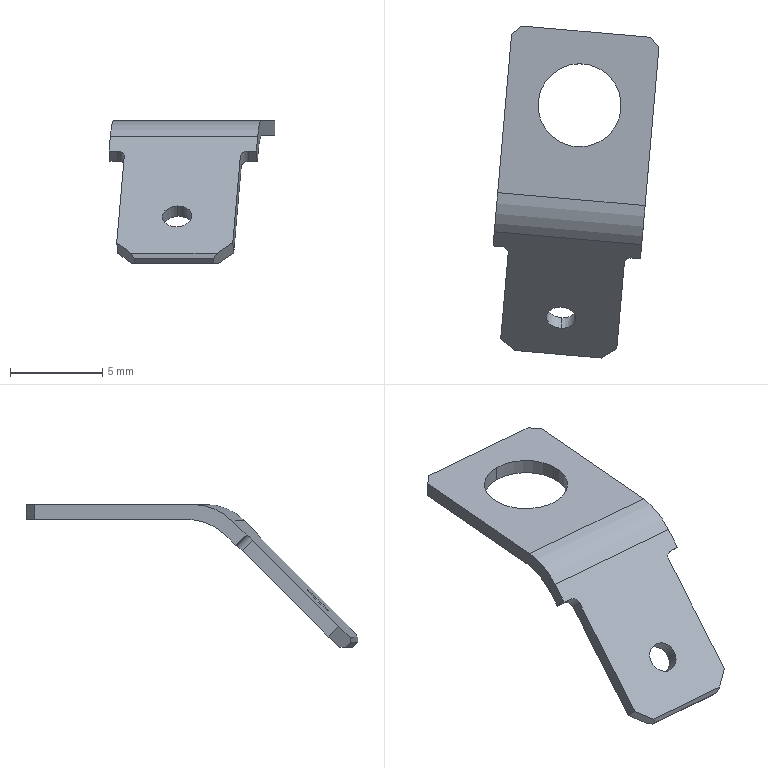Part | STEP file | MSBR-14_1_1_1_1 | 1 solid | 26 faces | box 8.97 x 17.939 x 7.73 mm | volume 103.786 mm3 | plane 18 | cylinder 8 | commonest cylinder face diameters 0.8 x2 1.6 x2 4.5 x2 6 x2
STEP:
#1=CARTESIAN_POINT('',(0.,0.,0.));
#2=DIRECTION('',(0.,0.,1.));
#3=DIRECTION('',(1.,0.,0.));
#4=AXIS2_PLACEMENT_3D('',#1,#2,#3);
#5=CARTESIAN_POINT('',(32.173,-29.923,38.));
#6=VERTEX_POINT('',#5);
#7=CARTESIAN_POINT('',(32.173,-29.923,38.8));
#8=VERTEX_POINT('',#7);
#9=CARTESIAN_POINT('',(32.173,-29.923,38.));
#10=DIRECTION('',(0.,0.,1.));
#11=VECTOR('',#10,0.8);
#12=LINE('',#9,#11);
#13=EDGE_CURVE('',#6,#8,#12,.T.);
#14=ORIENTED_EDGE('',*,*,#13,.F.);
#15=CARTESIAN_POINT('',(32.173,-34.423,38.));
#16=VERTEX_POINT('',#15);
#17=CARTESIAN_POINT('',(32.173,-32.173,38.));
#18=DIRECTION('',(0.,0.,-1.));
#19=DIRECTION('',(0.,-1.,0.));
#20=AXIS2_PLACEMENT_3D('',#17,#18,#19);
#21=CIRCLE('',#20,2.25);
#22=EDGE_CURVE('',#16,#6,#21,.T.);
#23=ORIENTED_EDGE('',*,*,#22,.F.);
#24=CARTESIAN_POINT('',(32.173,-34.423,38.8));
#25=VERTEX_POINT('',#24);
#26=CARTESIAN_POINT('',(32.173,-34.423,38.8));
#27=DIRECTION('',(0.,0.,-1.));
#28=VECTOR('',#27,0.8);
#29=LINE('',#26,#28);
#30=EDGE_CURVE('',#25,#16,#29,.T.);
#31=ORIENTED_EDGE('',*,*,#30,.F.);
#32=CARTESIAN_POINT('',(32.173,-32.173,38.8));
#33=DIRECTION('',(0.,0.,1.));
#34=DIRECTION('',(0.,1.,0.));
#35=AXIS2_PLACEMENT_3D('',#32,#33,#34);
#36=CIRCLE('',#35,2.25);
#37=EDGE_CURVE('',#8,#25,#36,.T.);
#38=ORIENTED_EDGE('',*,*,#37,.F.);
#39=EDGE_LOOP('',(#14,#23,#31,#38));
#40=FACE_OUTER_BOUND('',#39,.F.);
#41=CARTESIAN_POINT('',(32.173,-32.173,38.826));
#42=DIRECTION('',(0.,0.,-1.));
#43=DIRECTION('',(0.,-1.,0.));
#44=AXIS2_PLACEMENT_3D('',#41,#42,#43);
#45=CYLINDRICAL_SURFACE('',#44,2.25);
#46=ADVANCED_FACE('',(#40),#45,.F.);
#47=CARTESIAN_POINT('',(32.173,-32.173,38.));
#48=DIRECTION('',(0.,0.,-1.));
#49=DIRECTION('',(0.,1.,0.));
#50=AXIS2_PLACEMENT_3D('',#47,#48,#49);
#51=CIRCLE('',#50,2.25);
#52=EDGE_CURVE('',#6,#16,#51,.T.);
#53=ORIENTED_EDGE('',*,*,#52,.F.);
#54=ORIENTED_EDGE('',*,*,#13,.T.);
#55=CARTESIAN_POINT('',(32.173,-32.173,38.8));
#56=DIRECTION('',(0.,0.,1.));
#57=DIRECTION('',(0.,-1.,0.));
#58=AXIS2_PLACEMENT_3D('',#55,#56,#57);
#59=CIRCLE('',#58,2.25);
#60=EDGE_CURVE('',#25,#8,#59,.T.);
#61=ORIENTED_EDGE('',*,*,#60,.F.);
#62=ORIENTED_EDGE('',*,*,#30,.T.);
#63=EDGE_LOOP('',(#53,#54,#61,#62));
#64=FACE_OUTER_BOUND('',#63,.F.);
#65=CARTESIAN_POINT('',(32.173,-32.173,38.826));
#66=DIRECTION('',(0.,0.,-1.));
#67=DIRECTION('',(0.,1.,0.));
#68=AXIS2_PLACEMENT_3D('',#65,#66,#67);
#69=CYLINDRICAL_SURFACE('',#68,2.25);
#70=ADVANCED_FACE('',(#64),#69,.F.);
#71=CARTESIAN_POINT('',(35.744,-37.261,38.));
#72=VERTEX_POINT('',#71);
#73=CARTESIAN_POINT('',(27.774,-36.564,38.));
#74=VERTEX_POINT('',#73);
#75=CARTESIAN_POINT('',(35.744,-37.261,38.));
#76=DIRECTION('',(-0.9962,0.08716,0.));
#77=VECTOR('',#76,8.);
#78=LINE('',#75,#77);
#79=EDGE_CURVE('',#72,#74,#78,.T.);
#80=ORIENTED_EDGE('',*,*,#79,.F.);
#81=CARTESIAN_POINT('',(36.463,-29.035,38.));
#82=VERTEX_POINT('',#81);
#83=CARTESIAN_POINT('',(36.463,-29.035,38.));
#84=DIRECTION('',(-0.08716,-0.9962,0.));
#85=VECTOR('',#84,8.257);
#86=LINE('',#83,#85);
#87=EDGE_CURVE('',#82,#72,#86,.T.);
#88=ORIENTED_EDGE('',*,*,#87,.F.);
#89=CARTESIAN_POINT('',(36.009,-28.494,38.));
#90=VERTEX_POINT('',#89);
#91=CARTESIAN_POINT('',(36.463,-29.035,38.));
#92=DIRECTION('',(-0.6428,0.766,0.));
#93=VECTOR('',#92,0.7071);
#94=LINE('',#91,#93);
#95=EDGE_CURVE('',#82,#90,#94,.T.);
#96=ORIENTED_EDGE('',*,*,#95,.T.);
#97=CARTESIAN_POINT('',(29.035,-27.884,38.));
#98=VERTEX_POINT('',#97);
#99=CARTESIAN_POINT('',(29.035,-27.884,38.));
#100=DIRECTION('',(0.9962,-0.08716,0.));
#101=VECTOR('',#100,7.);
#102=LINE('',#99,#101);
#103=EDGE_CURVE('',#98,#90,#102,.T.);
#104=ORIENTED_EDGE('',*,*,#103,.F.);
#105=CARTESIAN_POINT('',(28.494,-28.338,38.));
#106=VERTEX_POINT('',#105);
#107=CARTESIAN_POINT('',(29.035,-27.884,38.));
#108=DIRECTION('',(-0.766,-0.6428,0.));
#109=VECTOR('',#108,0.7071);
#110=LINE('',#107,#109);
#111=EDGE_CURVE('',#98,#106,#110,.T.);
#112=ORIENTED_EDGE('',*,*,#111,.T.);
#113=CARTESIAN_POINT('',(27.774,-36.564,38.));
#114=DIRECTION('',(0.08716,0.9962,0.));
#115=VECTOR('',#114,8.257);
#116=LINE('',#113,#115);
#117=EDGE_CURVE('',#74,#106,#116,.T.);
#118=ORIENTED_EDGE('',*,*,#117,.F.);
#119=EDGE_LOOP('',(#80,#88,#96,#104,#112,#118));
#120=FACE_OUTER_BOUND('',#119,.F.);
#121=ORIENTED_EDGE('',*,*,#22,.T.);
#122=ORIENTED_EDGE('',*,*,#52,.T.);
#123=EDGE_LOOP('',(#121,#122));
#124=FACE_BOUND('',#123,.F.);
#125=CARTESIAN_POINT('',(32.14,-32.551,38.));
#126=DIRECTION('',(0.,0.,1.));
#127=DIRECTION('',(-0.08716,-0.9962,0.));
#128=AXIS2_PLACEMENT_3D('',#125,#126,#127);
#129=PLANE('',#128);
#130=ADVANCED_FACE('',(#120,#124),#129,.F.);
#131=ORIENTED_EDGE('',*,*,#79,.T.);
#132=CARTESIAN_POINT('',(27.589,-38.677,37.121));
#133=VERTEX_POINT('',#132);
#134=CARTESIAN_POINT('',(27.774,-36.564,35.));
#135=DIRECTION('',(-0.9962,0.08716,0.));
#136=DIRECTION('',(-0.06163,-0.7044,0.7071));
#137=AXIS2_PLACEMENT_3D('',#134,#135,#136);
#138=CIRCLE('',#137,3.);
#139=EDGE_CURVE('',#133,#74,#138,.T.);
#140=ORIENTED_EDGE('',*,*,#139,.F.);
#141=CARTESIAN_POINT('',(35.559,-39.374,37.121));
#142=VERTEX_POINT('',#141);
#143=CARTESIAN_POINT('',(27.589,-38.677,37.121));
#144=DIRECTION('',(0.9962,-0.08716,-0.000000002));
#145=VECTOR('',#144,8.);
#146=LINE('',#143,#145);
#147=EDGE_CURVE('',#133,#142,#146,.T.);
#148=ORIENTED_EDGE('',*,*,#147,.T.);
#149=CARTESIAN_POINT('',(35.744,-37.261,35.));
#150=DIRECTION('',(0.9962,-0.08716,0.));
#151=DIRECTION('',(0.000000003,0.000000023,1.));
#152=AXIS2_PLACEMENT_3D('',#149,#150,#151);
#153=CIRCLE('',#152,3.);
#154=EDGE_CURVE('',#72,#142,#153,.T.);
#155=ORIENTED_EDGE('',*,*,#154,.F.);
#156=EDGE_LOOP('',(#131,#140,#148,#155));
#157=FACE_OUTER_BOUND('',#156,.F.);
#158=CARTESIAN_POINT('',(35.903,-37.275,35.));
#159=DIRECTION('',(-0.9962,0.08716,0.));
#160=DIRECTION('',(-0.06163,-0.7044,0.7071));
#161=AXIS2_PLACEMENT_3D('',#158,#159,#160);
#162=CYLINDRICAL_SURFACE('',#161,3.);
#163=ADVANCED_FACE('',(#157),#162,.F.);
#164=CARTESIAN_POINT('',(27.745,-36.894,38.8));
#165=VERTEX_POINT('',#164);
#166=CARTESIAN_POINT('',(27.56,-39.007,37.921));
#167=VERTEX_POINT('',#166);
#168=CARTESIAN_POINT('',(27.745,-36.894,35.8));
#169=DIRECTION('',(0.9962,-0.08716,0.));
#170=DIRECTION('',(-0.000000002,-0.000000023,1.));
#171=AXIS2_PLACEMENT_3D('',#168,#169,#170);
#172=CIRCLE('',#171,3.);
#173=EDGE_CURVE('',#165,#167,#172,.T.);
#174=ORIENTED_EDGE('',*,*,#173,.T.);
#175=CARTESIAN_POINT('',(27.493,-39.774,37.151));
#176=VERTEX_POINT('',#175);
#177=CARTESIAN_POINT('',(27.56,-39.007,37.921));
#178=DIRECTION('',(-0.06163,-0.7044,-0.7071));
#179=VECTOR('',#178,1.089);
#180=LINE('',#177,#179);
#181=EDGE_CURVE('',#167,#176,#180,.T.);
#182=ORIENTED_EDGE('',*,*,#181,.T.);
#183=CARTESIAN_POINT('',(27.542,-39.211,36.586));
#184=VERTEX_POINT('',#183);
#185=CARTESIAN_POINT('',(27.493,-39.774,37.151));
#186=DIRECTION('',(0.06163,0.7044,-0.7071));
#187=VECTOR('',#186,0.8);
#188=LINE('',#185,#187);
#189=EDGE_CURVE('',#176,#184,#188,.T.);
#190=ORIENTED_EDGE('',*,*,#189,.T.);
#191=CARTESIAN_POINT('',(27.542,-39.211,36.586));
#192=DIRECTION('',(0.06163,0.7044,0.7071));
#193=VECTOR('',#192,0.7574);
#194=LINE('',#191,#193);
#195=EDGE_CURVE('',#184,#133,#194,.T.);
#196=ORIENTED_EDGE('',*,*,#195,.T.);
#197=ORIENTED_EDGE('',*,*,#139,.T.);
#198=ORIENTED_EDGE('',*,*,#117,.T.);
#199=CARTESIAN_POINT('',(28.494,-28.338,38.8));
#200=VERTEX_POINT('',#199);
#201=CARTESIAN_POINT('',(28.494,-28.338,38.8));
#202=DIRECTION('',(0.,0.,-1.));
#203=VECTOR('',#202,0.8);
#204=LINE('',#201,#203);
#205=EDGE_CURVE('',#200,#106,#204,.T.);
#206=ORIENTED_EDGE('',*,*,#205,.F.);
#207=CARTESIAN_POINT('',(27.745,-36.894,38.8));
#208=DIRECTION('',(0.08716,0.9962,0.));
#209=VECTOR('',#208,8.589);
#210=LINE('',#207,#209);
#211=EDGE_CURVE('',#165,#200,#210,.T.);
#212=ORIENTED_EDGE('',*,*,#211,.F.);
#213=EDGE_LOOP('',(#174,#182,#190,#196,#197,#198,#206,#212));
#214=FACE_OUTER_BOUND('',#213,.F.);
#215=CARTESIAN_POINT('',(27.993,-34.056,37.693));
#216=DIRECTION('',(0.9962,-0.08716,0.));
#217=DIRECTION('',(0.08716,0.9962,0.));
#218=AXIS2_PLACEMENT_3D('',#215,#216,#217);
#219=PLANE('',#218);
#220=ADVANCED_FACE('',(#214),#219,.F.);
#221=CARTESIAN_POINT('',(35.53,-39.705,37.921));
#222=VERTEX_POINT('',#221);
#223=CARTESIAN_POINT('',(35.715,-37.591,38.8));
#224=VERTEX_POINT('',#223);
#225=CARTESIAN_POINT('',(35.715,-37.591,35.8));
#226=DIRECTION('',(-0.9962,0.08716,0.));
#227=DIRECTION('',(-0.06163,-0.7044,0.7071));
#228=AXIS2_PLACEMENT_3D('',#225,#226,#227);
#229=CIRCLE('',#228,3.);
#230=EDGE_CURVE('',#222,#224,#229,.T.);
#231=ORIENTED_EDGE('',*,*,#230,.F.);
#232=CARTESIAN_POINT('',(35.53,-39.705,37.921));
#233=DIRECTION('',(-0.9962,0.08716,0.000000002));
#234=VECTOR('',#233,8.);
#235=LINE('',#232,#234);
#236=EDGE_CURVE('',#222,#167,#235,.T.);
#237=ORIENTED_EDGE('',*,*,#236,.T.);
#238=ORIENTED_EDGE('',*,*,#173,.F.);
#239=CARTESIAN_POINT('',(27.745,-36.894,38.8));
#240=DIRECTION('',(0.9962,-0.08716,0.));
#241=VECTOR('',#240,8.);
#242=LINE('',#239,#241);
#243=EDGE_CURVE('',#165,#224,#242,.T.);
#244=ORIENTED_EDGE('',*,*,#243,.T.);
#245=EDGE_LOOP('',(#231,#237,#238,#244));
#246=FACE_OUTER_BOUND('',#245,.F.);
#247=CARTESIAN_POINT('',(27.586,-36.88,35.8));
#248=DIRECTION('',(0.9962,-0.08716,0.));
#249=DIRECTION('',(0.,0.,1.));
#250=AXIS2_PLACEMENT_3D('',#247,#248,#249);
#251=CYLINDRICAL_SURFACE('',#250,3.);
#252=ADVANCED_FACE('',(#246),#251,.T.);
#253=CARTESIAN_POINT('',(35.512,-39.908,36.586));
#254=VERTEX_POINT('',#253);
#255=CARTESIAN_POINT('',(35.463,-40.472,37.151));
#256=VERTEX_POINT('',#255);
#257=CARTESIAN_POINT('',(35.512,-39.908,36.586));
#258=DIRECTION('',(-0.06163,-0.7044,0.7071));
#259=VECTOR('',#258,0.8);
#260=LINE('',#257,#259);
#261=EDGE_CURVE('',#254,#256,#260,.T.);
#262=ORIENTED_EDGE('',*,*,#261,.T.);
#263=CARTESIAN_POINT('',(35.463,-40.472,37.151));
#264=DIRECTION('',(0.06163,0.7044,0.7071));
#265=VECTOR('',#264,1.089);
#266=LINE('',#263,#265);
#267=EDGE_CURVE('',#256,#222,#266,.T.);
#268=ORIENTED_EDGE('',*,*,#267,.T.);
#269=ORIENTED_EDGE('',*,*,#230,.T.);
#270=CARTESIAN_POINT('',(36.463,-29.035,38.8));
#271=VERTEX_POINT('',#270);
#272=CARTESIAN_POINT('',(36.463,-29.035,38.8));
#273=DIRECTION('',(-0.08716,-0.9962,0.));
#274=VECTOR('',#273,8.589);
#275=LINE('',#272,#274);
#276=EDGE_CURVE('',#271,#224,#275,.T.);
#277=ORIENTED_EDGE('',*,*,#276,.F.);
#278=CARTESIAN_POINT('',(36.463,-29.035,38.));
#279=DIRECTION('',(0.,0.,1.));
#280=VECTOR('',#279,0.8);
#281=LINE('',#278,#280);
#282=EDGE_CURVE('',#82,#271,#281,.T.);
#283=ORIENTED_EDGE('',*,*,#282,.F.);
#284=ORIENTED_EDGE('',*,*,#87,.T.);
#285=ORIENTED_EDGE('',*,*,#154,.T.);
#286=CARTESIAN_POINT('',(35.559,-39.374,37.121));
#287=DIRECTION('',(-0.06163,-0.7044,-0.7071));
#288=VECTOR('',#287,0.7574);
#289=LINE('',#286,#288);
#290=EDGE_CURVE('',#142,#254,#289,.T.);
#291=ORIENTED_EDGE('',*,*,#290,.T.);
#292=EDGE_LOOP('',(#262,#268,#269,#277,#283,#284,#285,#291));
#293=FACE_OUTER_BOUND('',#292,.F.);
#294=CARTESIAN_POINT('',(35.963,-34.753,37.693));
#295=DIRECTION('',(0.9962,-0.08716,0.));
#296=DIRECTION('',(0.08716,0.9962,0.));
#297=AXIS2_PLACEMENT_3D('',#294,#295,#296);
#298=PLANE('',#297);
#299=ADVANCED_FACE('',(#293),#298,.T.);
#300=ORIENTED_EDGE('',*,*,#261,.F.);
#301=CARTESIAN_POINT('',(35.064,-39.869,36.586));
#302=VERTEX_POINT('',#301);
#303=CARTESIAN_POINT('',(35.064,-39.869,36.586));
#304=DIRECTION('',(0.9962,-0.08716,0.));
#305=VECTOR('',#304,0.45);
#306=LINE('',#303,#305);
#307=EDGE_CURVE('',#302,#254,#306,.T.);
#308=ORIENTED_EDGE('',*,*,#307,.F.);
#309=CARTESIAN_POINT('',(35.014,-40.432,37.151));
#310=VERTEX_POINT('',#309);
#311=CARTESIAN_POINT('',(35.014,-40.432,37.151));
#312=DIRECTION('',(0.06163,0.7044,-0.7071));
#313=VECTOR('',#312,0.8);
#314=LINE('',#311,#313);
#315=EDGE_CURVE('',#310,#302,#314,.T.);
#316=ORIENTED_EDGE('',*,*,#315,.F.);
#317=CARTESIAN_POINT('',(35.463,-40.472,37.151));
#318=DIRECTION('',(-0.9962,0.08716,0.));
#319=VECTOR('',#318,0.45);
#320=LINE('',#317,#319);
#321=EDGE_CURVE('',#256,#310,#320,.T.);
#322=ORIENTED_EDGE('',*,*,#321,.F.);
#323=EDGE_LOOP('',(#300,#308,#316,#322));
#324=FACE_OUTER_BOUND('',#323,.F.);
#325=CARTESIAN_POINT('',(35.263,-40.17,36.869));
#326=DIRECTION('',(0.06163,0.7044,0.7071));
#327=DIRECTION('',(0.9962,-0.08716,0.));
#328=AXIS2_PLACEMENT_3D('',#325,#326,#327);
#329=PLANE('',#328);
#330=ADVANCED_FACE('',(#324),#329,.F.);
#331=ORIENTED_EDGE('',*,*,#147,.F.);
#332=ORIENTED_EDGE('',*,*,#195,.F.);
#333=CARTESIAN_POINT('',(27.991,-39.25,36.586));
#334=VERTEX_POINT('',#333);
#335=CARTESIAN_POINT('',(27.991,-39.25,36.586));
#336=DIRECTION('',(-0.9962,0.08716,0.));
#337=VECTOR('',#336,0.45);
#338=LINE('',#335,#337);
#339=EDGE_CURVE('',#334,#184,#338,.T.);
#340=ORIENTED_EDGE('',*,*,#339,.F.);
#341=CARTESIAN_POINT('',(28.365,-39.567,36.303));
#342=VERTEX_POINT('',#341);
#343=CARTESIAN_POINT('',(27.966,-39.532,36.303));
#344=DIRECTION('',(0.06163,0.7044,-0.7071));
#345=DIRECTION('',(0.06163,0.7044,0.7071));
#346=AXIS2_PLACEMENT_3D('',#343,#344,#345);
#347=CIRCLE('',#346,0.4);
#348=EDGE_CURVE('',#334,#342,#347,.T.);
#349=ORIENTED_EDGE('',*,*,#348,.T.);
#350=CARTESIAN_POINT('',(27.958,-44.216,31.636));
#351=VERTEX_POINT('',#350);
#352=CARTESIAN_POINT('',(27.958,-44.216,31.636));
#353=DIRECTION('',(0.06163,0.7044,0.7071));
#354=VECTOR('',#353,6.6);
#355=LINE('',#352,#354);
#356=EDGE_CURVE('',#351,#342,#355,.T.);
#357=ORIENTED_EDGE('',*,*,#356,.F.);
#358=CARTESIAN_POINT('',(28.705,-44.849,31.07));
#359=VERTEX_POINT('',#358);
#360=CARTESIAN_POINT('',(28.705,-44.849,31.07));
#361=DIRECTION('',(-0.6608,0.5597,0.5));
#362=VECTOR('',#361,1.131);
#363=LINE('',#360,#362);
#364=EDGE_CURVE('',#359,#351,#363,.T.);
#365=ORIENTED_EDGE('',*,*,#364,.F.);
#366=CARTESIAN_POINT('',(33.388,-45.259,31.07));
#367=VERTEX_POINT('',#366);
#368=CARTESIAN_POINT('',(33.388,-45.259,31.07));
#369=DIRECTION('',(-0.9962,0.08716,0.));
#370=VECTOR('',#369,4.7);
#371=LINE('',#368,#370);
#372=EDGE_CURVE('',#367,#359,#371,.T.);
#373=ORIENTED_EDGE('',*,*,#372,.F.);
#374=CARTESIAN_POINT('',(34.234,-44.765,31.636));
#375=VERTEX_POINT('',#374);
#376=CARTESIAN_POINT('',(34.234,-44.765,31.636));
#377=DIRECTION('',(-0.748,-0.4365,-0.5));
#378=VECTOR('',#377,1.131);
#379=LINE('',#376,#378);
#380=EDGE_CURVE('',#375,#367,#379,.T.);
#381=ORIENTED_EDGE('',*,*,#380,.F.);
#382=CARTESIAN_POINT('',(34.641,-40.116,36.303));
#383=VERTEX_POINT('',#382);
#384=CARTESIAN_POINT('',(34.641,-40.116,36.303));
#385=DIRECTION('',(-0.06163,-0.7044,-0.7071));
#386=VECTOR('',#385,6.6);
#387=LINE('',#384,#386);
#388=EDGE_CURVE('',#383,#375,#387,.T.);
#389=ORIENTED_EDGE('',*,*,#388,.F.);
#390=CARTESIAN_POINT('',(35.039,-40.151,36.303));
#391=DIRECTION('',(0.06163,0.7044,-0.7071));
#392=DIRECTION('',(-0.9962,0.08716,-0.000000007));
#393=AXIS2_PLACEMENT_3D('',#390,#391,#392);
#394=CIRCLE('',#393,0.4);
#395=EDGE_CURVE('',#383,#302,#394,.T.);
#396=ORIENTED_EDGE('',*,*,#395,.T.);
#397=ORIENTED_EDGE('',*,*,#307,.T.);
#398=ORIENTED_EDGE('',*,*,#290,.F.);
#399=EDGE_LOOP('',(#331,#332,#340,#349,#357,#365,#373,#381,#389,#396,#397,#398));
#400=FACE_OUTER_BOUND('',#399,.F.);
#401=CARTESIAN_POINT('',(31.219,-42.515,33.615));
#402=VERTEX_POINT('',#401);
#403=CARTESIAN_POINT('',(31.219,-43.648,32.486));
#404=VERTEX_POINT('',#403);
#405=CARTESIAN_POINT('',(31.219,-43.081,33.05));
#406=DIRECTION('',(0.06163,0.7044,-0.7071));
#407=DIRECTION('',(0.000000001,0.7085,0.7058));
#408=AXIS2_PLACEMENT_3D('',#405,#406,#407);
#409=CIRCLE('',#408,0.8);
#410=EDGE_CURVE('',#402,#404,#409,.T.);
#411=ORIENTED_EDGE('',*,*,#410,.T.);
#412=CARTESIAN_POINT('',(31.219,-43.081,33.05));
#413=DIRECTION('',(0.06163,0.7044,-0.7071));
#414=DIRECTION('',(-0.000000002,-0.7085,-0.7058));
#415=AXIS2_PLACEMENT_3D('',#412,#413,#414);
#416=CIRCLE('',#415,0.8);
#417=EDGE_CURVE('',#404,#402,#416,.T.);
#418=ORIENTED_EDGE('',*,*,#417,.T.);
#419=EDGE_LOOP('',(#411,#418));
#420=FACE_BOUND('',#419,.F.);
#421=CARTESIAN_POINT('',(31.31,-42.04,34.096));
#422=DIRECTION('',(0.06163,0.7044,-0.7071));
#423=DIRECTION('',(-0.06163,-0.7044,-0.7071));
#424=AXIS2_PLACEMENT_3D('',#421,#422,#423);
#425=PLANE('',#424);
#426=ADVANCED_FACE('',(#400,#420),#425,.T.);
#427=ORIENTED_EDGE('',*,*,#189,.F.);
#428=CARTESIAN_POINT('',(27.941,-39.813,37.151));
#429=VERTEX_POINT('',#428);
#430=CARTESIAN_POINT('',(27.941,-39.813,37.151));
#431=DIRECTION('',(-0.9962,0.08716,0.000000001));
#432=VECTOR('',#431,0.45);
#433=LINE('',#430,#432);
#434=EDGE_CURVE('',#429,#176,#433,.T.);
#435=ORIENTED_EDGE('',*,*,#434,.F.);
#436=CARTESIAN_POINT('',(27.991,-39.25,36.586));
#437=DIRECTION('',(-0.06163,-0.7044,0.7071));
#438=VECTOR('',#437,0.8);
#439=LINE('',#436,#438);
#440=EDGE_CURVE('',#334,#429,#439,.T.);
#441=ORIENTED_EDGE('',*,*,#440,.F.);
#442=ORIENTED_EDGE('',*,*,#339,.T.);
#443=EDGE_LOOP('',(#427,#435,#441,#442));
#444=FACE_OUTER_BOUND('',#443,.F.);
#445=CARTESIAN_POINT('',(27.742,-39.512,36.869));
#446=DIRECTION('',(0.06163,0.7044,0.7071));
#447=DIRECTION('',(0.9962,-0.08716,0.));
#448=AXIS2_PLACEMENT_3D('',#445,#446,#447);
#449=PLANE('',#448);
#450=ADVANCED_FACE('',(#444),#449,.F.);
#451=ORIENTED_EDGE('',*,*,#434,.T.);
#452=ORIENTED_EDGE('',*,*,#181,.F.);
#453=ORIENTED_EDGE('',*,*,#236,.F.);
#454=ORIENTED_EDGE('',*,*,#267,.F.);
#455=ORIENTED_EDGE('',*,*,#321,.T.);
#456=CARTESIAN_POINT('',(34.591,-40.679,36.869));
#457=VERTEX_POINT('',#456);
#458=CARTESIAN_POINT('',(34.99,-40.714,36.869));
#459=DIRECTION('',(-0.06163,-0.7044,0.7071));
#460=DIRECTION('',(0.06163,0.7044,0.7071));
#461=AXIS2_PLACEMENT_3D('',#458,#459,#460);
#462=CIRCLE('',#461,0.4);
#463=EDGE_CURVE('',#310,#457,#462,.T.);
#464=ORIENTED_EDGE('',*,*,#463,.T.);
#465=CARTESIAN_POINT('',(34.184,-45.328,32.202));
#466=VERTEX_POINT('',#465);
#467=CARTESIAN_POINT('',(34.184,-45.328,32.202));
#468=DIRECTION('',(0.06163,0.7044,0.7071));
#469=VECTOR('',#468,6.6);
#470=LINE('',#467,#469);
#471=EDGE_CURVE('',#466,#457,#470,.T.);
#472=ORIENTED_EDGE('',*,*,#471,.F.);
#473=CARTESIAN_POINT('',(33.338,-45.822,31.636));
#474=VERTEX_POINT('',#473);
#475=CARTESIAN_POINT('',(33.338,-45.822,31.636));
#476=DIRECTION('',(0.748,0.4365,0.5));
#477=VECTOR('',#476,1.131);
#478=LINE('',#475,#477);
#479=EDGE_CURVE('',#474,#466,#478,.T.);
#480=ORIENTED_EDGE('',*,*,#479,.F.);
#481=CARTESIAN_POINT('',(28.656,-45.413,31.636));
#482=VERTEX_POINT('',#481);
#483=CARTESIAN_POINT('',(28.656,-45.413,31.636));
#484=DIRECTION('',(0.9962,-0.08716,0.));
#485=VECTOR('',#484,4.7);
#486=LINE('',#483,#485);
#487=EDGE_CURVE('',#482,#474,#486,.T.);
#488=ORIENTED_EDGE('',*,*,#487,.F.);
#489=CARTESIAN_POINT('',(27.908,-44.779,32.202));
#490=VERTEX_POINT('',#489);
#491=CARTESIAN_POINT('',(27.908,-44.779,32.202));
#492=DIRECTION('',(0.6608,-0.5597,-0.5));
#493=VECTOR('',#492,1.131);
#494=LINE('',#491,#493);
#495=EDGE_CURVE('',#490,#482,#494,.T.);
#496=ORIENTED_EDGE('',*,*,#495,.F.);
#497=CARTESIAN_POINT('',(28.315,-40.13,36.869));
#498=VERTEX_POINT('',#497);
#499=CARTESIAN_POINT('',(28.315,-40.13,36.869));
#500=DIRECTION('',(-0.06163,-0.7044,-0.7071));
#501=VECTOR('',#500,6.6);
#502=LINE('',#499,#501);
#503=EDGE_CURVE('',#498,#490,#502,.T.);
#504=ORIENTED_EDGE('',*,*,#503,.F.);
#505=CARTESIAN_POINT('',(27.917,-40.095,36.869));
#506=DIRECTION('',(-0.06163,-0.7044,0.7071));
#507=DIRECTION('',(0.9962,-0.08716,-0.000000036));
#508=AXIS2_PLACEMENT_3D('',#505,#506,#507);
#509=CIRCLE('',#508,0.4);
#510=EDGE_CURVE('',#498,#429,#509,.T.);
#511=ORIENTED_EDGE('',*,*,#510,.T.);
#512=EDGE_LOOP('',(#451,#452,#453,#454,#455,#464,#472,#480,#488,#496,#504,#511));
#513=FACE_OUTER_BOUND('',#512,.F.);
#514=CARTESIAN_POINT('',(31.17,-43.078,34.181));
#515=VERTEX_POINT('',#514);
#516=CARTESIAN_POINT('',(31.17,-44.212,33.051));
#517=VERTEX_POINT('',#516);
#518=CARTESIAN_POINT('',(31.17,-43.645,33.616));
#519=DIRECTION('',(-0.06163,-0.7044,0.7071));
#520=DIRECTION('',(-0.000000001,0.7085,0.7058));
#521=AXIS2_PLACEMENT_3D('',#518,#519,#520);
#522=CIRCLE('',#521,0.8);
#523=EDGE_CURVE('',#515,#517,#522,.T.);
#524=ORIENTED_EDGE('',*,*,#523,.T.);
#525=CARTESIAN_POINT('',(31.17,-43.645,33.616));
#526=DIRECTION('',(-0.06163,-0.7044,0.7071));
#527=DIRECTION('',(0.000000001,-0.7085,-0.7058));
#528=AXIS2_PLACEMENT_3D('',#525,#526,#527);
#529=CIRCLE('',#528,0.8);
#530=EDGE_CURVE('',#517,#515,#529,.T.);
#531=ORIENTED_EDGE('',*,*,#530,.T.);
#532=EDGE_LOOP('',(#524,#531));
#533=FACE_BOUND('',#532,.F.);
#534=CARTESIAN_POINT('',(31.271,-42.487,34.779));
#535=DIRECTION('',(0.06163,0.7044,-0.7071));
#536=DIRECTION('',(0.06163,0.7044,0.7071));
#537=AXIS2_PLACEMENT_3D('',#534,#535,#536);
#538=PLANE('',#537);
#539=ADVANCED_FACE('',(#513,#533),#538,.F.);
#540=CARTESIAN_POINT('',(34.641,-40.116,36.303));
#541=DIRECTION('',(-0.06163,-0.7044,0.7071));
#542=VECTOR('',#541,0.8);
#543=LINE('',#540,#542);
#544=EDGE_CURVE('',#383,#457,#543,.T.);
#545=ORIENTED_EDGE('',*,*,#544,.T.);
#546=ORIENTED_EDGE('',*,*,#463,.F.);
#547=ORIENTED_EDGE('',*,*,#315,.T.);
#548=ORIENTED_EDGE('',*,*,#395,.F.);
#549=EDGE_LOOP('',(#545,#546,#547,#548));
#550=FACE_OUTER_BOUND('',#549,.F.);
#551=CARTESIAN_POINT('',(35.041,-40.132,36.284));
#552=DIRECTION('',(-0.06163,-0.7044,0.7071));
#553=DIRECTION('',(0.06163,0.7044,0.7071));
#554=AXIS2_PLACEMENT_3D('',#551,#552,#553);
#555=CYLINDRICAL_SURFACE('',#554,0.4);
#556=ADVANCED_FACE('',(#550),#555,.F.);
#557=CARTESIAN_POINT('',(34.184,-45.328,32.202));
#558=DIRECTION('',(0.06163,0.7044,-0.7071));
#559=VECTOR('',#558,0.8);
#560=LINE('',#557,#559);
#561=EDGE_CURVE('',#466,#375,#560,.T.);
#562=ORIENTED_EDGE('',*,*,#561,.F.);
#563=ORIENTED_EDGE('',*,*,#471,.T.);
#564=ORIENTED_EDGE('',*,*,#544,.F.);
#565=ORIENTED_EDGE('',*,*,#388,.T.);
#566=EDGE_LOOP('',(#562,#563,#564,#565));
#567=FACE_OUTER_BOUND('',#566,.F.);
#568=CARTESIAN_POINT('',(34.413,-42.722,34.252));
#569=DIRECTION('',(0.9962,-0.08716,0.));
#570=DIRECTION('',(0.06163,0.7044,0.7071));
#571=AXIS2_PLACEMENT_3D('',#568,#569,#570);
#572=PLANE('',#571);
#573=ADVANCED_FACE('',(#567),#572,.T.);
#574=ORIENTED_EDGE('',*,*,#561,.T.);
#575=ORIENTED_EDGE('',*,*,#380,.T.);
#576=CARTESIAN_POINT('',(33.164,-45.523,31.07));
#577=VERTEX_POINT('',#576);
#578=CARTESIAN_POINT('',(33.164,-45.523,31.07));
#579=DIRECTION('',(0.6463,0.7631,0.));
#580=VECTOR('',#579,0.3464);
#581=LINE('',#578,#580);
#582=EDGE_CURVE('',#577,#367,#581,.T.);
#583=ORIENTED_EDGE('',*,*,#582,.F.);
#584=CARTESIAN_POINT('',(33.139,-45.805,31.353));
#585=VERTEX_POINT('',#584);
#586=CARTESIAN_POINT('',(33.164,-45.523,31.07));
#587=DIRECTION('',(-0.06163,-0.7044,0.7071));
#588=VECTOR('',#587,0.4);
#589=LINE('',#586,#588);
#590=EDGE_CURVE('',#577,#585,#589,.T.);
#591=ORIENTED_EDGE('',*,*,#590,.T.);
#592=CARTESIAN_POINT('',(33.338,-45.822,31.636));
#593=DIRECTION('',(-0.5752,0.05032,-0.8165));
#594=VECTOR('',#593,0.3464);
#595=LINE('',#592,#594);
#596=EDGE_CURVE('',#474,#585,#595,.T.);
#597=ORIENTED_EDGE('',*,*,#596,.F.);
#598=ORIENTED_EDGE('',*,*,#479,.T.);
#599=EDGE_LOOP('',(#574,#575,#583,#591,#597,#598));
#600=FACE_OUTER_BOUND('',#599,.F.);
#601=CARTESIAN_POINT('',(33.749,-45.338,31.636));
#602=DIRECTION('',(0.6608,-0.5597,-0.5));
#603=DIRECTION('',(0.3815,-0.3232,0.866));
#604=AXIS2_PLACEMENT_3D('',#601,#602,#603);
#605=PLANE('',#604);
#606=ADVANCED_FACE('',(#600),#605,.T.);
#607=ORIENTED_EDGE('',*,*,#582,.T.);
#608=ORIENTED_EDGE('',*,*,#372,.T.);
#609=CARTESIAN_POINT('',(28.88,-45.148,31.07));
#610=VERTEX_POINT('',#609);
#611=CARTESIAN_POINT('',(28.705,-44.849,31.07));
#612=DIRECTION('',(0.504,-0.8637,-0.000000001));
#613=VECTOR('',#612,0.3464);
#614=LINE('',#611,#613);
#615=EDGE_CURVE('',#359,#610,#614,.T.);
#616=ORIENTED_EDGE('',*,*,#615,.T.);
#617=CARTESIAN_POINT('',(33.164,-45.523,31.07));
#618=DIRECTION('',(-0.9962,0.08716,0.));
#619=VECTOR('',#618,4.3);
#620=LINE('',#617,#619);
#621=EDGE_CURVE('',#577,#610,#620,.T.);
#622=ORIENTED_EDGE('',*,*,#621,.F.);
#623=EDGE_LOOP('',(#607,#608,#616,#622));
#624=FACE_OUTER_BOUND('',#623,.F.);
#625=CARTESIAN_POINT('',(31.034,-45.195,31.07));
#626=DIRECTION('',(0.,0.,1.));
#627=DIRECTION('',(0.9962,-0.08716,0.));
#628=AXIS2_PLACEMENT_3D('',#625,#626,#627);
#629=PLANE('',#628);
#630=ADVANCED_FACE('',(#624),#629,.F.);
#631=ORIENTED_EDGE('',*,*,#615,.F.);
#632=ORIENTED_EDGE('',*,*,#364,.T.);
#633=CARTESIAN_POINT('',(27.958,-44.216,31.636));
#634=DIRECTION('',(-0.06163,-0.7044,0.7071));
#635=VECTOR('',#634,0.8);
#636=LINE('',#633,#635);
#637=EDGE_CURVE('',#351,#490,#636,.T.);
#638=ORIENTED_EDGE('',*,*,#637,.T.);
#639=ORIENTED_EDGE('',*,*,#495,.T.);
#640=CARTESIAN_POINT('',(28.855,-45.43,31.353));
#641=VERTEX_POINT('',#640);
#642=CARTESIAN_POINT('',(28.855,-45.43,31.353));
#643=DIRECTION('',(-0.5752,0.05032,0.8165));
#644=VECTOR('',#643,0.3464);
#645=LINE('',#642,#644);
#646=EDGE_CURVE('',#641,#482,#645,.T.);
#647=ORIENTED_EDGE('',*,*,#646,.F.);
#648=CARTESIAN_POINT('',(28.855,-45.43,31.353));
#649=DIRECTION('',(0.06163,0.7044,-0.7071));
#650=VECTOR('',#649,0.4);
#651=LINE('',#648,#650);
#652=EDGE_CURVE('',#641,#610,#651,.T.);
#653=ORIENTED_EDGE('',*,*,#652,.T.);
#654=EDGE_LOOP('',(#631,#632,#638,#639,#647,#653));
#655=FACE_OUTER_BOUND('',#654,.F.);
#656=CARTESIAN_POINT('',(28.336,-44.864,31.636));
#657=DIRECTION('',(0.748,0.4365,0.5));
#658=DIRECTION('',(-0.4319,-0.252,0.866));
#659=AXIS2_PLACEMENT_3D('',#656,#657,#658);
#660=PLANE('',#659);
#661=ADVANCED_FACE('',(#655),#660,.F.);
#662=CARTESIAN_POINT('',(28.315,-40.13,36.869));
#663=DIRECTION('',(0.06163,0.7044,-0.7071));
#664=VECTOR('',#663,0.8);
#665=LINE('',#662,#664);
#666=EDGE_CURVE('',#498,#342,#665,.T.);
#667=ORIENTED_EDGE('',*,*,#666,.F.);
#668=ORIENTED_EDGE('',*,*,#503,.T.);
#669=ORIENTED_EDGE('',*,*,#637,.F.);
#670=ORIENTED_EDGE('',*,*,#356,.T.);
#671=EDGE_LOOP('',(#667,#668,#669,#670));
#672=FACE_OUTER_BOUND('',#671,.F.);
#673=CARTESIAN_POINT('',(28.136,-42.173,34.252));
#674=DIRECTION('',(0.9962,-0.08716,0.));
#675=DIRECTION('',(-0.06163,-0.7044,-0.7071));
#676=AXIS2_PLACEMENT_3D('',#673,#674,#675);
#677=PLANE('',#676);
#678=ADVANCED_FACE('',(#672),#677,.F.);
#679=ORIENTED_EDGE('',*,*,#440,.T.);
#680=ORIENTED_EDGE('',*,*,#510,.F.);
#681=ORIENTED_EDGE('',*,*,#666,.T.);
#682=ORIENTED_EDGE('',*,*,#348,.F.);
#683=EDGE_LOOP('',(#679,#680,#681,#682));
#684=FACE_OUTER_BOUND('',#683,.F.);
#685=CARTESIAN_POINT('',(27.968,-39.513,36.284));
#686=DIRECTION('',(-0.06163,-0.7044,0.7071));
#687=DIRECTION('',(0.9962,-0.08716,0.000000002));
#688=AXIS2_PLACEMENT_3D('',#685,#686,#687);
#689=CYLINDRICAL_SURFACE('',#688,0.4);
#690=ADVANCED_FACE('',(#684),#689,.F.);
#691=ORIENTED_EDGE('',*,*,#596,.T.);
#692=CARTESIAN_POINT('',(28.855,-45.43,31.353));
#693=DIRECTION('',(0.9962,-0.08716,0.));
#694=VECTOR('',#693,4.3);
#695=LINE('',#692,#694);
#696=EDGE_CURVE('',#641,#585,#695,.T.);
#697=ORIENTED_EDGE('',*,*,#696,.F.);
#698=ORIENTED_EDGE('',*,*,#646,.T.);
#699=ORIENTED_EDGE('',*,*,#487,.T.);
#700=EDGE_LOOP('',(#691,#697,#698,#699));
#701=FACE_OUTER_BOUND('',#700,.F.);
#702=CARTESIAN_POINT('',(30.997,-45.617,31.495));
#703=DIRECTION('',(0.08716,0.9962,0.));
#704=DIRECTION('',(0.9962,-0.08716,0.));
#705=AXIS2_PLACEMENT_3D('',#702,#703,#704);
#706=PLANE('',#705);
#707=ADVANCED_FACE('',(#701),#706,.F.);
#708=ORIENTED_EDGE('',*,*,#621,.T.);
#709=ORIENTED_EDGE('',*,*,#652,.F.);
#710=ORIENTED_EDGE('',*,*,#696,.T.);
#711=ORIENTED_EDGE('',*,*,#590,.F.);
#712=EDGE_LOOP('',(#708,#709,#710,#711));
#713=FACE_OUTER_BOUND('',#712,.F.);
#714=CARTESIAN_POINT('',(31.009,-45.476,31.212));
#715=DIRECTION('',(0.06163,0.7044,0.7071));
#716=DIRECTION('',(-0.06163,-0.7044,0.7071));
#717=AXIS2_PLACEMENT_3D('',#714,#715,#716);
#718=PLANE('',#717);
#719=ADVANCED_FACE('',(#713),#718,.F.);
#720=ORIENTED_EDGE('',*,*,#523,.F.);
#721=CARTESIAN_POINT('',(31.219,-42.515,33.615));
#722=DIRECTION('',(-0.06163,-0.7044,0.7071));
#723=VECTOR('',#722,0.8);
#724=LINE('',#721,#723);
#725=EDGE_CURVE('',#402,#515,#724,.T.);
#726=ORIENTED_EDGE('',*,*,#725,.F.);
#727=ORIENTED_EDGE('',*,*,#417,.F.);
#728=CARTESIAN_POINT('',(31.17,-44.212,33.051));
#729=DIRECTION('',(0.06163,0.7044,-0.7071));
#730=VECTOR('',#729,0.8);
#731=LINE('',#728,#730);
#732=EDGE_CURVE('',#517,#404,#731,.T.);
#733=ORIENTED_EDGE('',*,*,#732,.F.);
#734=EDGE_LOOP('',(#720,#726,#727,#733));
#735=FACE_OUTER_BOUND('',#734,.F.);
#736=CARTESIAN_POINT('',(31.168,-43.664,33.635));
#737=DIRECTION('',(0.06163,0.7044,-0.7071));
#738=DIRECTION('',(-0.000000001,-0.7085,-0.7058));
#739=AXIS2_PLACEMENT_3D('',#736,#737,#738);
#740=CYLINDRICAL_SURFACE('',#739,0.8);
#741=ADVANCED_FACE('',(#735),#740,.F.);
#742=ORIENTED_EDGE('',*,*,#732,.T.);
#743=ORIENTED_EDGE('',*,*,#410,.F.);
#744=ORIENTED_EDGE('',*,*,#725,.T.);
#745=ORIENTED_EDGE('',*,*,#530,.F.);
#746=EDGE_LOOP('',(#742,#743,#744,#745));
#747=FACE_OUTER_BOUND('',#746,.F.);
#748=CARTESIAN_POINT('',(31.168,-43.664,33.635));
#749=DIRECTION('',(0.06163,0.7044,-0.7071));
#750=DIRECTION('',(0.,0.7085,0.7058));
#751=AXIS2_PLACEMENT_3D('',#748,#749,#750);
#752=CYLINDRICAL_SURFACE('',#751,0.8);
#753=ADVANCED_FACE('',(#747),#752,.F.);
#754=CARTESIAN_POINT('',(36.009,-28.494,38.8));
#755=VERTEX_POINT('',#754);
#756=CARTESIAN_POINT('',(36.009,-28.494,38.8));
#757=DIRECTION('',(0.6428,-0.766,0.));
#758=VECTOR('',#757,0.7071);
#759=LINE('',#756,#758);
#760=EDGE_CURVE('',#755,#271,#759,.T.);
#761=ORIENTED_EDGE('',*,*,#760,.T.);
#762=ORIENTED_EDGE('',*,*,#276,.T.);
#763=ORIENTED_EDGE('',*,*,#243,.F.);
#764=ORIENTED_EDGE('',*,*,#211,.T.);
#765=CARTESIAN_POINT('',(29.035,-27.884,38.8));
#766=VERTEX_POINT('',#765);
#767=CARTESIAN_POINT('',(28.494,-28.338,38.8));
#768=DIRECTION('',(0.766,0.6428,0.));
#769=VECTOR('',#768,0.7071);
#770=LINE('',#767,#769);
#771=EDGE_CURVE('',#200,#766,#770,.T.);
#772=ORIENTED_EDGE('',*,*,#771,.T.);
#773=CARTESIAN_POINT('',(36.009,-28.494,38.8));
#774=DIRECTION('',(-0.9962,0.08716,0.));
#775=VECTOR('',#774,7.);
#776=LINE('',#773,#775);
#777=EDGE_CURVE('',#755,#766,#776,.T.);
#778=ORIENTED_EDGE('',*,*,#777,.F.);
#779=EDGE_LOOP('',(#761,#762,#763,#764,#772,#778));
#780=FACE_OUTER_BOUND('',#779,.F.);
#781=ORIENTED_EDGE('',*,*,#37,.T.);
#782=ORIENTED_EDGE('',*,*,#60,.T.);
#783=EDGE_LOOP('',(#781,#782));
#784=FACE_BOUND('',#783,.F.);
#785=CARTESIAN_POINT('',(32.126,-32.716,38.8));
#786=DIRECTION('',(0.,0.,1.));
#787=DIRECTION('',(0.08716,0.9962,0.));
#788=AXIS2_PLACEMENT_3D('',#785,#786,#787);
#789=PLANE('',#788);
#790=ADVANCED_FACE('',(#780,#784),#789,.T.);
#791=ORIENTED_EDGE('',*,*,#95,.F.);
#792=ORIENTED_EDGE('',*,*,#282,.T.);
#793=ORIENTED_EDGE('',*,*,#760,.F.);
#794=CARTESIAN_POINT('',(36.009,-28.494,38.));
#795=DIRECTION('',(0.,0.,1.));
#796=VECTOR('',#795,0.8);
#797=LINE('',#794,#796);
#798=EDGE_CURVE('',#90,#755,#797,.T.);
#799=ORIENTED_EDGE('',*,*,#798,.F.);
#800=EDGE_LOOP('',(#791,#792,#793,#799));
#801=FACE_OUTER_BOUND('',#800,.F.);
#802=CARTESIAN_POINT('',(36.236,-28.764,38.4));
#803=DIRECTION('',(0.766,0.6428,0.));
#804=DIRECTION('',(0.,0.,1.));
#805=AXIS2_PLACEMENT_3D('',#802,#803,#804);
#806=PLANE('',#805);
#807=ADVANCED_FACE('',(#801),#806,.T.);
#808=CARTESIAN_POINT('',(29.035,-27.884,38.));
#809=DIRECTION('',(0.,0.,1.));
#810=VECTOR('',#809,0.8);
#811=LINE('',#808,#810);
#812=EDGE_CURVE('',#98,#766,#811,.T.);
#813=ORIENTED_EDGE('',*,*,#812,.F.);
#814=ORIENTED_EDGE('',*,*,#103,.T.);
#815=ORIENTED_EDGE('',*,*,#798,.T.);
#816=ORIENTED_EDGE('',*,*,#777,.T.);
#817=EDGE_LOOP('',(#813,#814,#815,#816));
#818=FACE_OUTER_BOUND('',#817,.F.);
#819=CARTESIAN_POINT('',(32.522,-28.189,38.4));
#820=DIRECTION('',(0.08716,0.9962,0.));
#821=DIRECTION('',(0.,0.,-1.));
#822=AXIS2_PLACEMENT_3D('',#819,#820,#821);
#823=PLANE('',#822);
#824=ADVANCED_FACE('',(#818),#823,.T.);
#825=ORIENTED_EDGE('',*,*,#111,.F.);
#826=ORIENTED_EDGE('',*,*,#812,.T.);
#827=ORIENTED_EDGE('',*,*,#771,.F.);
#828=ORIENTED_EDGE('',*,*,#205,.T.);
#829=EDGE_LOOP('',(#825,#826,#827,#828));
#830=FACE_OUTER_BOUND('',#829,.F.);
#831=CARTESIAN_POINT('',(28.764,-28.111,38.4));
#832=DIRECTION('',(-0.6428,0.766,0.));
#833=DIRECTION('',(0.,0.,1.));
#834=AXIS2_PLACEMENT_3D('',#831,#832,#833);
#835=PLANE('',#834);
#836=ADVANCED_FACE('',(#830),#835,.T.);
#837=CLOSED_SHELL('',(#46,#70,#130,#163,#220,#252,#299,#330,#426,#450,#539,#556,#573,#606,#630,#661,#678,#690,#707,#719,#741,#753,#790,#807,#824,#836));
#838=MANIFOLD_SOLID_BREP('',#837);
#839=(LENGTH_UNIT()NAMED_UNIT(*)SI_UNIT(.MILLI.,.METRE.));
#840=UNCERTAINTY_MEASURE_WITH_UNIT(LENGTH_MEASURE(0.0022),#839,'','');
#841=(NAMED_UNIT(*)PLANE_ANGLE_UNIT()SI_UNIT($,.RADIAN.));
#842=PLANE_ANGLE_MEASURE_WITH_UNIT(PLANE_ANGLE_MEASURE(0.01745),#841);
#843=(CONVERSION_BASED_UNIT('DEGREE',#842)NAMED_UNIT(*)PLANE_ANGLE_UNIT());
#844=(NAMED_UNIT(*)SI_UNIT($,.STERADIAN.)SOLID_ANGLE_UNIT());
#845=(GEOMETRIC_REPRESENTATION_CONTEXT(3)GLOBAL_UNCERTAINTY_ASSIGNED_CONTEXT((#840))GLOBAL_UNIT_ASSIGNED_CONTEXT((#839,#843,#844))REPRESENTATION_CONTEXT('',''));
#846=ADVANCED_BREP_SHAPE_REPRESENTATION('',(#4,#838),#845);